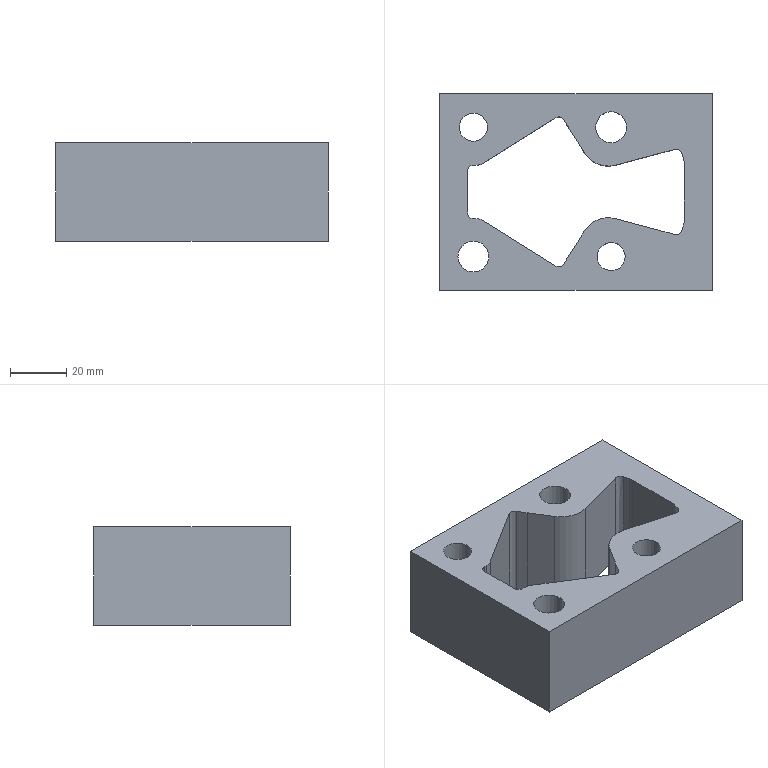Part | NX | features solid 2 | 1 solid | 44 faces | box 97 x 70 x 35 mm | volume 138939 mm3 | plane 20 | cylinder 18 | spline 6 | commonest cylinder face diameters 10 x6 4 x4 11 x2 12 x2 17 x2 20 x2
STEP:
#1=CARTESIAN_POINT('',(1528.396,23.,78.));
#2=VERTEX_POINT('',#1);
#3=CARTESIAN_POINT('',(1533.396,23.,78.));
#4=DIRECTION('',(0.,0.,-1.));
#5=DIRECTION('',(-1.,0.,0.));
#6=AXIS2_PLACEMENT_3D('',#3,#4,#5);
#7=CIRCLE('',#6,5.);
#8=EDGE_CURVE('',#2,#2,#7,.T.);
#9=ORIENTED_EDGE('',*,*,#8,.T.);
#10=EDGE_LOOP('',(#9));
#11=FACE_BOUND('',#10,.T.);
#12=CARTESIAN_POINT('',(1576.896,23.,78.));
#13=VERTEX_POINT('',#12);
#14=CARTESIAN_POINT('',(1582.396,23.,78.));
#15=DIRECTION('',(0.,0.,1.));
#16=DIRECTION('',(-1.,0.,0.));
#17=AXIS2_PLACEMENT_3D('',#14,#15,#16);
#18=CIRCLE('',#17,5.5);
#19=EDGE_CURVE('',#13,#13,#18,.F.);
#20=ORIENTED_EDGE('',*,*,#19,.T.);
#21=EDGE_LOOP('',(#20));
#22=FACE_BOUND('',#21,.T.);
#23=CARTESIAN_POINT('',(1577.396,-23.,78.));
#24=VERTEX_POINT('',#23);
#25=CARTESIAN_POINT('',(1582.396,-23.,78.));
#26=DIRECTION('',(0.,0.,-1.));
#27=DIRECTION('',(-1.,0.,0.));
#28=AXIS2_PLACEMENT_3D('',#25,#26,#27);
#29=CIRCLE('',#28,5.);
#30=EDGE_CURVE('',#24,#24,#29,.T.);
#31=ORIENTED_EDGE('',*,*,#30,.T.);
#32=EDGE_LOOP('',(#31));
#33=FACE_BOUND('',#32,.T.);
#34=CARTESIAN_POINT('',(1538.896,-23.,78.));
#35=VERTEX_POINT('',#34);
#36=CARTESIAN_POINT('',(1533.396,-23.,78.));
#37=DIRECTION('',(0.,0.,1.));
#38=DIRECTION('',(1.,0.,0.));
#39=AXIS2_PLACEMENT_3D('',#36,#37,#38);
#40=CIRCLE('',#39,5.5);
#41=EDGE_CURVE('',#35,#35,#40,.T.);
#42=ORIENTED_EDGE('',*,*,#41,.F.);
#43=EDGE_LOOP('',(#42));
#44=FACE_BOUND('',#43,.T.);
#45=CARTESIAN_POINT('',(1618.396,-35.,78.));
#46=VERTEX_POINT('',#45);
#47=CARTESIAN_POINT('',(1521.396,-35.,78.));
#48=VERTEX_POINT('',#47);
#49=CARTESIAN_POINT('',(1569.896,-35.,78.));
#50=DIRECTION('',(1.,0.,0.));
#51=VECTOR('',#50,1000.);
#52=LINE('',#49,#51);
#53=EDGE_CURVE('',#46,#48,#52,.F.);
#54=ORIENTED_EDGE('',*,*,#53,.F.);
#55=CARTESIAN_POINT('',(1618.396,35.,78.));
#56=VERTEX_POINT('',#55);
#57=CARTESIAN_POINT('',(1618.396,0.,78.));
#58=DIRECTION('',(0.,1.,0.));
#59=VECTOR('',#58,1000.);
#60=LINE('',#57,#59);
#61=EDGE_CURVE('',#56,#46,#60,.F.);
#62=ORIENTED_EDGE('',*,*,#61,.F.);
#63=CARTESIAN_POINT('',(1521.396,35.,78.));
#64=VERTEX_POINT('',#63);
#65=CARTESIAN_POINT('',(1569.896,35.,78.));
#66=DIRECTION('',(-1.,0.,0.));
#67=VECTOR('',#66,1000.);
#68=LINE('',#65,#67);
#69=EDGE_CURVE('',#64,#56,#68,.F.);
#70=ORIENTED_EDGE('',*,*,#69,.F.);
#71=CARTESIAN_POINT('',(1521.396,0.,78.));
#72=DIRECTION('',(0.,-1.,0.));
#73=VECTOR('',#72,1000.);
#74=LINE('',#71,#73);
#75=EDGE_CURVE('',#48,#64,#74,.F.);
#76=ORIENTED_EDGE('',*,*,#75,.F.);
#77=EDGE_LOOP('',(#54,#62,#70,#76));
#78=FACE_BOUND('',#77,.T.);
#79=CARTESIAN_POINT('',(1536.976,-10.26,78.));
#80=VERTEX_POINT('',#79);
#81=CARTESIAN_POINT('',(1534.327,-9.5,78.));
#82=VERTEX_POINT('',#81);
#83=CARTESIAN_POINT('',(1534.327,-14.5,78.));
#84=DIRECTION('',(0.,0.,-1.));
#85=DIRECTION('',(-1.,0.,0.));
#86=AXIS2_PLACEMENT_3D('',#83,#84,#85);
#87=CIRCLE('',#86,5.);
#88=EDGE_CURVE('',#80,#82,#87,.F.);
#89=ORIENTED_EDGE('',*,*,#88,.T.);
#90=CARTESIAN_POINT('',(1533.396,-9.5,78.));
#91=VERTEX_POINT('',#90);
#92=CARTESIAN_POINT('',(984.466,-9.5,78.));
#93=DIRECTION('',(-1.,0.,0.));
#94=VECTOR('',#93,1000.);
#95=LINE('',#92,#94);
#96=EDGE_CURVE('',#82,#91,#95,.T.);
#97=ORIENTED_EDGE('',*,*,#96,.T.);
#98=CARTESIAN_POINT('',(1531.396,-7.5,78.));
#99=VERTEX_POINT('',#98);
#100=CARTESIAN_POINT('',(1533.396,-7.5,78.));
#101=DIRECTION('',(0.,0.,-1.));
#102=DIRECTION('',(-1.,0.,0.));
#103=AXIS2_PLACEMENT_3D('',#100,#101,#102);
#104=CIRCLE('',#103,2.);
#105=EDGE_CURVE('',#91,#99,#104,.T.);
#106=ORIENTED_EDGE('',*,*,#105,.T.);
#107=CARTESIAN_POINT('',(1531.396,7.5,78.));
#108=VERTEX_POINT('',#107);
#109=CARTESIAN_POINT('',(1531.396,0.,78.));
#110=DIRECTION('',(0.,-1.,0.));
#111=VECTOR('',#110,1000.);
#112=LINE('',#109,#111);
#113=EDGE_CURVE('',#108,#99,#112,.T.);
#114=ORIENTED_EDGE('',*,*,#113,.F.);
#115=CARTESIAN_POINT('',(1533.396,9.5,78.));
#116=VERTEX_POINT('',#115);
#117=CARTESIAN_POINT('',(1533.396,7.5,78.));
#118=DIRECTION('',(0.,0.,-1.));
#119=DIRECTION('',(-1.,0.,0.));
#120=AXIS2_PLACEMENT_3D('',#117,#118,#119);
#121=CIRCLE('',#120,2.);
#122=EDGE_CURVE('',#116,#108,#121,.F.);
#123=ORIENTED_EDGE('',*,*,#122,.F.);
#124=CARTESIAN_POINT('',(1534.327,9.5,78.));
#125=VERTEX_POINT('',#124);
#126=CARTESIAN_POINT('',(2186.158,9.5,78.));
#127=DIRECTION('',(-1.,0.,0.));
#128=VECTOR('',#127,1000.);
#129=LINE('',#126,#128);
#130=EDGE_CURVE('',#125,#116,#129,.T.);
#131=ORIENTED_EDGE('',*,*,#130,.F.);
#132=CARTESIAN_POINT('',(1536.976,10.26,78.));
#133=VERTEX_POINT('',#132);
#134=CARTESIAN_POINT('',(1534.327,14.5,78.));
#135=DIRECTION('',(0.,0.,-1.));
#136=DIRECTION('',(-1.,0.,0.));
#137=AXIS2_PLACEMENT_3D('',#134,#135,#136);
#138=CIRCLE('',#137,5.);
#139=EDGE_CURVE('',#133,#125,#138,.T.);
#140=ORIENTED_EDGE('',*,*,#139,.F.);
#141=CARTESIAN_POINT('',(1562.757,26.369,78.));
#142=VERTEX_POINT('',#141);
#143=CARTESIAN_POINT('',(1999.247,299.119,78.));
#144=DIRECTION('',(0.848,0.5299,0.));
#145=VECTOR('',#144,1000.);
#146=LINE('',#143,#145);
#147=EDGE_CURVE('',#142,#133,#146,.F.);
#148=ORIENTED_EDGE('',*,*,#147,.F.);
#149=CARTESIAN_POINT('',(1565.512,25.733,78.));
#150=VERTEX_POINT('',#149);
#151=CARTESIAN_POINT('',(1563.816,24.673,78.));
#152=DIRECTION('',(0.,0.,-1.));
#153=DIRECTION('',(-1.,0.,0.));
#154=AXIS2_PLACEMENT_3D('',#151,#152,#153);
#155=CIRCLE('',#154,2.);
#156=EDGE_CURVE('',#150,#142,#155,.F.);
#157=ORIENTED_EDGE('',*,*,#156,.F.);
#158=CARTESIAN_POINT('',(1567.632,22.341,78.));
#159=VERTEX_POINT('',#158);
#160=CARTESIAN_POINT('',(1567.632,22.341,78.));
#161=DIRECTION('',(-0.5299,0.848,0.));
#162=VECTOR('',#161,1000.);
#163=LINE('',#160,#162);
#164=EDGE_CURVE('',#150,#159,#163,.F.);
#165=ORIENTED_EDGE('',*,*,#164,.T.);
#166=CARTESIAN_POINT('',(1572.931,13.86,78.));
#167=VERTEX_POINT('',#166);
#168=CARTESIAN_POINT('',(1572.931,13.86,78.));
#169=CARTESIAN_POINT('',(1571.165,16.687,78.));
#170=CARTESIAN_POINT('',(1569.399,19.514,78.));
#171=CARTESIAN_POINT('',(1567.632,22.341,78.));
#172=B_SPLINE_CURVE_WITH_KNOTS('',3,(#168,#169,#170,#171),.UNSPECIFIED.,.F.,.F.,(4,4),(0.,0.01),.UNSPECIFIED.);
#173=EDGE_CURVE('',#167,#159,#172,.T.);
#174=ORIENTED_EDGE('',*,*,#173,.F.);
#175=CARTESIAN_POINT('',(1584.,9.5,78.));
#176=VERTEX_POINT('',#175);
#177=CARTESIAN_POINT('',(1581.412,19.159,78.));
#178=DIRECTION('',(0.,0.,-1.));
#179=DIRECTION('',(-1.,0.,0.));
#180=AXIS2_PLACEMENT_3D('',#177,#178,#179);
#181=CIRCLE('',#180,10.);
#182=EDGE_CURVE('',#176,#167,#181,.T.);
#183=ORIENTED_EDGE('',*,*,#182,.F.);
#184=CARTESIAN_POINT('',(1605.133,15.163,78.));
#185=VERTEX_POINT('',#184);
#186=CARTESIAN_POINT('',(1605.133,15.163,78.));
#187=CARTESIAN_POINT('',(1598.089,13.275,78.));
#188=CARTESIAN_POINT('',(1591.044,11.388,78.));
#189=CARTESIAN_POINT('',(1584.,9.5,78.));
#190=B_SPLINE_CURVE_WITH_KNOTS('',3,(#186,#187,#188,#189),.UNSPECIFIED.,.F.,.F.,(4,4),(0.,0.02188),.UNSPECIFIED.);
#191=EDGE_CURVE('',#185,#176,#190,.T.);
#192=ORIENTED_EDGE('',*,*,#191,.F.);
#193=CARTESIAN_POINT('',(1607.583,13.748,78.));
#194=VERTEX_POINT('',#193);
#195=CARTESIAN_POINT('',(1605.651,13.231,78.));
#196=DIRECTION('',(0.,0.,-1.));
#197=DIRECTION('',(-1.,0.,0.));
#198=AXIS2_PLACEMENT_3D('',#195,#196,#197);
#199=CIRCLE('',#198,2.);
#200=EDGE_CURVE('',#194,#185,#199,.F.);
#201=ORIENTED_EDGE('',*,*,#200,.F.);
#202=CARTESIAN_POINT('',(1608.226,11.348,78.));
#203=VERTEX_POINT('',#202);
#204=CARTESIAN_POINT('',(1602.079,34.289,78.));
#205=DIRECTION('',(-0.2588,0.9659,0.));
#206=VECTOR('',#205,1000.);
#207=LINE('',#204,#206);
#208=EDGE_CURVE('',#194,#203,#207,.F.);
#209=ORIENTED_EDGE('',*,*,#208,.T.);
#210=CARTESIAN_POINT('',(1608.396,10.054,78.));
#211=VERTEX_POINT('',#210);
#212=CARTESIAN_POINT('',(1603.396,10.054,78.));
#213=DIRECTION('',(0.,0.,-1.));
#214=DIRECTION('',(-1.,0.,0.));
#215=AXIS2_PLACEMENT_3D('',#212,#213,#214);
#216=CIRCLE('',#215,5.);
#217=EDGE_CURVE('',#211,#203,#216,.F.);
#218=ORIENTED_EDGE('',*,*,#217,.F.);
#219=CARTESIAN_POINT('',(1608.396,-10.054,78.));
#220=VERTEX_POINT('',#219);
#221=CARTESIAN_POINT('',(1608.396,-4.33,78.));
#222=DIRECTION('',(0.,-1.,0.));
#223=VECTOR('',#222,1000.);
#224=LINE('',#221,#223);
#225=EDGE_CURVE('',#220,#211,#224,.F.);
#226=ORIENTED_EDGE('',*,*,#225,.F.);
#227=CARTESIAN_POINT('',(1608.226,-11.348,78.));
#228=VERTEX_POINT('',#227);
#229=CARTESIAN_POINT('',(1603.396,-10.054,78.));
#230=DIRECTION('',(0.,0.,-1.));
#231=DIRECTION('',(-1.,0.,0.));
#232=AXIS2_PLACEMENT_3D('',#229,#230,#231);
#233=CIRCLE('',#232,5.);
#234=EDGE_CURVE('',#220,#228,#233,.T.);
#235=ORIENTED_EDGE('',*,*,#234,.T.);
#236=CARTESIAN_POINT('',(1607.583,-13.748,78.));
#237=VERTEX_POINT('',#236);
#238=CARTESIAN_POINT('',(1602.079,-34.289,78.));
#239=DIRECTION('',(0.2588,0.9659,0.));
#240=VECTOR('',#239,1000.);
#241=LINE('',#238,#240);
#242=EDGE_CURVE('',#228,#237,#241,.F.);
#243=ORIENTED_EDGE('',*,*,#242,.T.);
#244=CARTESIAN_POINT('',(1605.133,-15.163,78.));
#245=VERTEX_POINT('',#244);
#246=CARTESIAN_POINT('',(1605.651,-13.231,78.));
#247=DIRECTION('',(0.,0.,-1.));
#248=DIRECTION('',(-1.,0.,0.));
#249=AXIS2_PLACEMENT_3D('',#246,#247,#248);
#250=CIRCLE('',#249,2.);
#251=EDGE_CURVE('',#237,#245,#250,.T.);
#252=ORIENTED_EDGE('',*,*,#251,.T.);
#253=CARTESIAN_POINT('',(1584.,-9.5,78.));
#254=VERTEX_POINT('',#253);
#255=CARTESIAN_POINT('',(1605.133,-15.163,78.));
#256=CARTESIAN_POINT('',(1598.089,-13.275,78.));
#257=CARTESIAN_POINT('',(1591.044,-11.388,78.));
#258=CARTESIAN_POINT('',(1584.,-9.5,78.));
#259=B_SPLINE_CURVE_WITH_KNOTS('',3,(#255,#256,#257,#258),.UNSPECIFIED.,.F.,.F.,(4,4),(0.,0.02188),.UNSPECIFIED.);
#260=EDGE_CURVE('',#245,#254,#259,.T.);
#261=ORIENTED_EDGE('',*,*,#260,.T.);
#262=CARTESIAN_POINT('',(1572.931,-13.86,78.));
#263=VERTEX_POINT('',#262);
#264=CARTESIAN_POINT('',(1581.412,-19.159,78.));
#265=DIRECTION('',(0.,0.,-1.));
#266=DIRECTION('',(-1.,0.,0.));
#267=AXIS2_PLACEMENT_3D('',#264,#265,#266);
#268=CIRCLE('',#267,10.);
#269=EDGE_CURVE('',#254,#263,#268,.F.);
#270=ORIENTED_EDGE('',*,*,#269,.T.);
#271=CARTESIAN_POINT('',(1567.632,-22.341,78.));
#272=VERTEX_POINT('',#271);
#273=CARTESIAN_POINT('',(1572.931,-13.86,78.));
#274=CARTESIAN_POINT('',(1571.165,-16.687,78.));
#275=CARTESIAN_POINT('',(1569.399,-19.514,78.));
#276=CARTESIAN_POINT('',(1567.632,-22.341,78.));
#277=B_SPLINE_CURVE_WITH_KNOTS('',3,(#273,#274,#275,#276),.UNSPECIFIED.,.F.,.F.,(4,4),(0.,0.01),.UNSPECIFIED.);
#278=EDGE_CURVE('',#263,#272,#277,.T.);
#279=ORIENTED_EDGE('',*,*,#278,.T.);
#280=CARTESIAN_POINT('',(1565.512,-25.733,78.));
#281=VERTEX_POINT('',#280);
#282=CARTESIAN_POINT('',(1751.363,271.69,78.));
#283=DIRECTION('',(-0.5299,-0.848,0.));
#284=VECTOR('',#283,1000.);
#285=LINE('',#282,#284);
#286=EDGE_CURVE('',#281,#272,#285,.F.);
#287=ORIENTED_EDGE('',*,*,#286,.F.);
#288=CARTESIAN_POINT('',(1562.757,-26.369,78.));
#289=VERTEX_POINT('',#288);
#290=CARTESIAN_POINT('',(1563.816,-24.673,78.));
#291=DIRECTION('',(0.,0.,-1.));
#292=DIRECTION('',(-1.,0.,0.));
#293=AXIS2_PLACEMENT_3D('',#290,#291,#292);
#294=CIRCLE('',#293,2.);
#295=EDGE_CURVE('',#281,#289,#294,.T.);
#296=ORIENTED_EDGE('',*,*,#295,.T.);
#297=CARTESIAN_POINT('',(1636.537,-72.472,78.));
#298=DIRECTION('',(0.848,-0.5299,0.));
#299=VECTOR('',#298,1000.);
#300=LINE('',#297,#299);
#301=EDGE_CURVE('',#289,#80,#300,.F.);
#302=ORIENTED_EDGE('',*,*,#301,.T.);
#303=EDGE_LOOP('',(#89,#97,#106,#114,#123,#131,#140,#148,#157,#165,#174,#183,#192,#201,#209,#218,#226,#235,#243,#252,#261,#270,#279,#287,#296,#302));
#304=FACE_BOUND('',#303,.T.);
#305=CARTESIAN_POINT('',(2186.158,0.000000688,78.));
#306=DIRECTION('',(0.,0.,-1.));
#307=DIRECTION('',(1.,0.,0.));
#308=AXIS2_PLACEMENT_3D('',#305,#306,#307);
#309=PLANE('',#308);
#310=ADVANCED_FACE('',(#11,#22,#33,#44,#78,#304),#309,.F.);
#311=CARTESIAN_POINT('',(1527.396,23.,43.));
#312=VERTEX_POINT('',#311);
#313=CARTESIAN_POINT('',(1533.396,23.,43.));
#314=DIRECTION('',(0.,0.,-1.));
#315=DIRECTION('',(-1.,0.,0.));
#316=AXIS2_PLACEMENT_3D('',#313,#314,#315);
#317=CIRCLE('',#316,6.);
#318=EDGE_CURVE('',#312,#312,#317,.F.);
#319=ORIENTED_EDGE('',*,*,#318,.F.);
#320=EDGE_LOOP('',(#319));
#321=FACE_BOUND('',#320,.T.);
#322=CARTESIAN_POINT('',(1539.396,23.,58.));
#323=VERTEX_POINT('',#322);
#324=CARTESIAN_POINT('',(1533.396,23.,58.));
#325=DIRECTION('',(0.,0.,1.));
#326=DIRECTION('',(1.,0.,0.));
#327=AXIS2_PLACEMENT_3D('',#324,#325,#326);
#328=CIRCLE('',#327,6.);
#329=EDGE_CURVE('',#323,#323,#328,.F.);
#330=ORIENTED_EDGE('',*,*,#329,.F.);
#331=EDGE_LOOP('',(#330));
#332=FACE_BOUND('',#331,.T.);
#333=CARTESIAN_POINT('',(1533.396,23.,43.));
#334=DIRECTION('',(0.,0.,1.));
#335=DIRECTION('',(1.,0.,0.));
#336=AXIS2_PLACEMENT_3D('',#333,#334,#335);
#337=CYLINDRICAL_SURFACE('',#336,6.);
#338=ADVANCED_FACE('',(#321,#332),#337,.F.);
#339=ORIENTED_EDGE('',*,*,#8,.F.);
#340=EDGE_LOOP('',(#339));
#341=FACE_BOUND('',#340,.T.);
#342=CARTESIAN_POINT('',(1538.396,23.,58.));
#343=VERTEX_POINT('',#342);
#344=CARTESIAN_POINT('',(1533.396,23.,58.));
#345=DIRECTION('',(0.,0.,1.));
#346=DIRECTION('',(1.,0.,0.));
#347=AXIS2_PLACEMENT_3D('',#344,#345,#346);
#348=CIRCLE('',#347,5.);
#349=EDGE_CURVE('',#343,#343,#348,.F.);
#350=ORIENTED_EDGE('',*,*,#349,.T.);
#351=EDGE_LOOP('',(#350));
#352=FACE_BOUND('',#351,.T.);
#353=CARTESIAN_POINT('',(1533.396,23.,78.));
#354=DIRECTION('',(0.,0.,1.));
#355=DIRECTION('',(1.,0.,0.));
#356=AXIS2_PLACEMENT_3D('',#353,#354,#355);
#357=CYLINDRICAL_SURFACE('',#356,5.);
#358=ADVANCED_FACE('',(#341,#352),#357,.F.);
#359=ORIENTED_EDGE('',*,*,#329,.T.);
#360=EDGE_LOOP('',(#359));
#361=FACE_BOUND('',#360,.T.);
#362=ORIENTED_EDGE('',*,*,#349,.F.);
#363=EDGE_LOOP('',(#362));
#364=FACE_BOUND('',#363,.T.);
#365=CARTESIAN_POINT('',(1531.574,23.49,58.));
#366=DIRECTION('',(0.,0.,1.));
#367=DIRECTION('',(1.,0.,0.));
#368=AXIS2_PLACEMENT_3D('',#365,#366,#367);
#369=PLANE('',#368);
#370=ADVANCED_FACE('',(#361,#364),#369,.F.);
#371=CARTESIAN_POINT('',(1573.896,23.,43.));
#372=VERTEX_POINT('',#371);
#373=CARTESIAN_POINT('',(1582.396,23.,43.));
#374=DIRECTION('',(0.,0.,1.));
#375=DIRECTION('',(-1.,0.,0.));
#376=AXIS2_PLACEMENT_3D('',#373,#374,#375);
#377=CIRCLE('',#376,8.5);
#378=EDGE_CURVE('',#372,#372,#377,.T.);
#379=ORIENTED_EDGE('',*,*,#378,.F.);
#380=EDGE_LOOP('',(#379));
#381=FACE_BOUND('',#380,.T.);
#382=CARTESIAN_POINT('',(1573.896,23.,58.));
#383=VERTEX_POINT('',#382);
#384=CARTESIAN_POINT('',(1582.396,23.,58.));
#385=DIRECTION('',(0.,0.,1.));
#386=DIRECTION('',(-1.,0.,0.));
#387=AXIS2_PLACEMENT_3D('',#384,#385,#386);
#388=CIRCLE('',#387,8.5);
#389=EDGE_CURVE('',#383,#383,#388,.F.);
#390=ORIENTED_EDGE('',*,*,#389,.F.);
#391=EDGE_LOOP('',(#390));
#392=FACE_BOUND('',#391,.T.);
#393=CARTESIAN_POINT('',(1582.396,23.,43.));
#394=DIRECTION('',(0.,0.,1.));
#395=DIRECTION('',(-1.,0.,0.));
#396=AXIS2_PLACEMENT_3D('',#393,#394,#395);
#397=CYLINDRICAL_SURFACE('',#396,8.5);
#398=ADVANCED_FACE('',(#381,#392),#397,.F.);
#399=ORIENTED_EDGE('',*,*,#19,.F.);
#400=EDGE_LOOP('',(#399));
#401=FACE_BOUND('',#400,.T.);
#402=CARTESIAN_POINT('',(1576.896,23.,58.));
#403=VERTEX_POINT('',#402);
#404=CARTESIAN_POINT('',(1582.396,23.,58.));
#405=DIRECTION('',(0.,0.,1.));
#406=DIRECTION('',(-1.,0.,0.));
#407=AXIS2_PLACEMENT_3D('',#404,#405,#406);
#408=CIRCLE('',#407,5.5);
#409=EDGE_CURVE('',#403,#403,#408,.F.);
#410=ORIENTED_EDGE('',*,*,#409,.T.);
#411=EDGE_LOOP('',(#410));
#412=FACE_BOUND('',#411,.T.);
#413=CARTESIAN_POINT('',(1582.396,23.,78.));
#414=DIRECTION('',(0.,0.,1.));
#415=DIRECTION('',(-1.,0.,0.));
#416=AXIS2_PLACEMENT_3D('',#413,#414,#415);
#417=CYLINDRICAL_SURFACE('',#416,5.5);
#418=ADVANCED_FACE('',(#401,#412),#417,.F.);
#419=ORIENTED_EDGE('',*,*,#389,.T.);
#420=EDGE_LOOP('',(#419));
#421=FACE_BOUND('',#420,.T.);
#422=ORIENTED_EDGE('',*,*,#409,.F.);
#423=EDGE_LOOP('',(#422));
#424=FACE_BOUND('',#423,.T.);
#425=CARTESIAN_POINT('',(1584.218,23.49,58.));
#426=DIRECTION('',(0.,0.,1.));
#427=DIRECTION('',(-1.,0.,0.));
#428=AXIS2_PLACEMENT_3D('',#425,#426,#427);
#429=PLANE('',#428);
#430=ADVANCED_FACE('',(#421,#424),#429,.F.);
#431=CARTESIAN_POINT('',(1541.896,-23.,58.));
#432=VERTEX_POINT('',#431);
#433=CARTESIAN_POINT('',(1533.396,-23.,58.));
#434=DIRECTION('',(0.,0.,1.));
#435=DIRECTION('',(1.,0.,0.));
#436=AXIS2_PLACEMENT_3D('',#433,#434,#435);
#437=CIRCLE('',#436,8.5);
#438=EDGE_CURVE('',#432,#432,#437,.F.);
#439=ORIENTED_EDGE('',*,*,#438,.T.);
#440=EDGE_LOOP('',(#439));
#441=FACE_BOUND('',#440,.T.);
#442=CARTESIAN_POINT('',(1538.896,-23.,58.));
#443=VERTEX_POINT('',#442);
#444=CARTESIAN_POINT('',(1533.396,-23.,58.));
#445=DIRECTION('',(0.,0.,1.));
#446=DIRECTION('',(1.,0.,0.));
#447=AXIS2_PLACEMENT_3D('',#444,#445,#446);
#448=CIRCLE('',#447,5.5);
#449=EDGE_CURVE('',#443,#443,#448,.F.);
#450=ORIENTED_EDGE('',*,*,#449,.F.);
#451=EDGE_LOOP('',(#450));
#452=FACE_BOUND('',#451,.T.);
#453=CARTESIAN_POINT('',(1531.574,-23.49,58.));
#454=DIRECTION('',(0.,0.,1.));
#455=DIRECTION('',(1.,0.,0.));
#456=AXIS2_PLACEMENT_3D('',#453,#454,#455);
#457=PLANE('',#456);
#458=ADVANCED_FACE('',(#441,#452),#457,.F.);
#459=CARTESIAN_POINT('',(1588.396,-23.,58.));
#460=VERTEX_POINT('',#459);
#461=CARTESIAN_POINT('',(1582.396,-23.,58.));
#462=DIRECTION('',(0.,0.,1.));
#463=DIRECTION('',(1.,0.,0.));
#464=AXIS2_PLACEMENT_3D('',#461,#462,#463);
#465=CIRCLE('',#464,6.);
#466=EDGE_CURVE('',#460,#460,#465,.F.);
#467=ORIENTED_EDGE('',*,*,#466,.T.);
#468=EDGE_LOOP('',(#467));
#469=FACE_BOUND('',#468,.T.);
#470=CARTESIAN_POINT('',(1587.396,-23.,58.));
#471=VERTEX_POINT('',#470);
#472=CARTESIAN_POINT('',(1582.396,-23.,58.));
#473=DIRECTION('',(0.,0.,1.));
#474=DIRECTION('',(1.,0.,0.));
#475=AXIS2_PLACEMENT_3D('',#472,#473,#474);
#476=CIRCLE('',#475,5.);
#477=EDGE_CURVE('',#471,#471,#476,.F.);
#478=ORIENTED_EDGE('',*,*,#477,.F.);
#479=EDGE_LOOP('',(#478));
#480=FACE_BOUND('',#479,.T.);
#481=CARTESIAN_POINT('',(1584.218,-23.49,58.));
#482=DIRECTION('',(0.,0.,1.));
#483=DIRECTION('',(-1.,0.,0.));
#484=AXIS2_PLACEMENT_3D('',#481,#482,#483);
#485=PLANE('',#484);
#486=ADVANCED_FACE('',(#469,#480),#485,.F.);
#487=CARTESIAN_POINT('',(1541.896,-23.,43.));
#488=VERTEX_POINT('',#487);
#489=CARTESIAN_POINT('',(1533.396,-23.,43.));
#490=DIRECTION('',(0.,0.,1.));
#491=DIRECTION('',(1.,0.,0.));
#492=AXIS2_PLACEMENT_3D('',#489,#490,#491);
#493=CIRCLE('',#492,8.5);
#494=EDGE_CURVE('',#488,#488,#493,.T.);
#495=ORIENTED_EDGE('',*,*,#494,.F.);
#496=EDGE_LOOP('',(#495));
#497=FACE_BOUND('',#496,.T.);
#498=ORIENTED_EDGE('',*,*,#438,.F.);
#499=EDGE_LOOP('',(#498));
#500=FACE_BOUND('',#499,.T.);
#501=CARTESIAN_POINT('',(1533.396,-23.,43.));
#502=DIRECTION('',(0.,0.,1.));
#503=DIRECTION('',(1.,0.,0.));
#504=AXIS2_PLACEMENT_3D('',#501,#502,#503);
#505=CYLINDRICAL_SURFACE('',#504,8.5);
#506=ADVANCED_FACE('',(#497,#500),#505,.F.);
#507=CARTESIAN_POINT('',(1521.396,-35.,43.));
#508=VERTEX_POINT('',#507);
#509=CARTESIAN_POINT('',(1521.396,-35.,22.));
#510=DIRECTION('',(0.,0.,1.));
#511=VECTOR('',#510,1000.);
#512=LINE('',#509,#511);
#513=EDGE_CURVE('',#508,#48,#512,.T.);
#514=ORIENTED_EDGE('',*,*,#513,.T.);
#515=ORIENTED_EDGE('',*,*,#75,.T.);
#516=CARTESIAN_POINT('',(1521.396,35.,43.));
#517=VERTEX_POINT('',#516);
#518=CARTESIAN_POINT('',(1521.396,35.,22.));
#519=DIRECTION('',(0.,0.,1.));
#520=VECTOR('',#519,1000.);
#521=LINE('',#518,#520);
#522=EDGE_CURVE('',#517,#64,#521,.T.);
#523=ORIENTED_EDGE('',*,*,#522,.F.);
#524=CARTESIAN_POINT('',(1521.396,0.,43.));
#525=DIRECTION('',(0.,-1.,0.));
#526=VECTOR('',#525,1000.);
#527=LINE('',#524,#526);
#528=EDGE_CURVE('',#517,#508,#527,.T.);
#529=ORIENTED_EDGE('',*,*,#528,.T.);
#530=EDGE_LOOP('',(#514,#515,#523,#529));
#531=FACE_BOUND('',#530,.T.);
#532=CARTESIAN_POINT('',(1521.396,0.,22.));
#533=DIRECTION('',(-1.,0.,0.));
#534=DIRECTION('',(0.,0.,1.));
#535=AXIS2_PLACEMENT_3D('',#532,#533,#534);
#536=PLANE('',#535);
#537=ADVANCED_FACE('',(#531),#536,.T.);
#538=ORIENTED_EDGE('',*,*,#522,.T.);
#539=ORIENTED_EDGE('',*,*,#69,.T.);
#540=CARTESIAN_POINT('',(1618.396,35.,43.));
#541=VERTEX_POINT('',#540);
#542=CARTESIAN_POINT('',(1618.396,35.,22.));
#543=DIRECTION('',(0.,0.,1.));
#544=VECTOR('',#543,1000.);
#545=LINE('',#542,#544);
#546=EDGE_CURVE('',#541,#56,#545,.T.);
#547=ORIENTED_EDGE('',*,*,#546,.F.);
#548=CARTESIAN_POINT('',(1569.896,35.,43.));
#549=DIRECTION('',(-1.,0.,0.));
#550=VECTOR('',#549,1000.);
#551=LINE('',#548,#550);
#552=EDGE_CURVE('',#541,#517,#551,.T.);
#553=ORIENTED_EDGE('',*,*,#552,.T.);
#554=EDGE_LOOP('',(#538,#539,#547,#553));
#555=FACE_BOUND('',#554,.T.);
#556=CARTESIAN_POINT('',(1569.896,35.,22.));
#557=DIRECTION('',(0.,1.,0.));
#558=DIRECTION('',(0.,0.,1.));
#559=AXIS2_PLACEMENT_3D('',#556,#557,#558);
#560=PLANE('',#559);
#561=ADVANCED_FACE('',(#555),#560,.T.);
#562=CARTESIAN_POINT('',(1618.396,-35.,43.));
#563=VERTEX_POINT('',#562);
#564=CARTESIAN_POINT('',(1618.396,0.,43.));
#565=DIRECTION('',(0.,1.,0.));
#566=VECTOR('',#565,1000.);
#567=LINE('',#564,#566);
#568=EDGE_CURVE('',#563,#541,#567,.T.);
#569=ORIENTED_EDGE('',*,*,#568,.T.);
#570=ORIENTED_EDGE('',*,*,#546,.T.);
#571=ORIENTED_EDGE('',*,*,#61,.T.);
#572=CARTESIAN_POINT('',(1618.396,-35.,22.));
#573=DIRECTION('',(0.,0.,1.));
#574=VECTOR('',#573,1000.);
#575=LINE('',#572,#574);
#576=EDGE_CURVE('',#563,#46,#575,.T.);
#577=ORIENTED_EDGE('',*,*,#576,.F.);
#578=EDGE_LOOP('',(#569,#570,#571,#577));
#579=FACE_BOUND('',#578,.T.);
#580=CARTESIAN_POINT('',(1618.396,0.,22.));
#581=DIRECTION('',(1.,0.,0.));
#582=DIRECTION('',(0.,0.,-1.));
#583=AXIS2_PLACEMENT_3D('',#580,#581,#582);
#584=PLANE('',#583);
#585=ADVANCED_FACE('',(#579),#584,.T.);
#586=ORIENTED_EDGE('',*,*,#513,.F.);
#587=CARTESIAN_POINT('',(1569.896,-35.,43.));
#588=DIRECTION('',(1.,0.,0.));
#589=VECTOR('',#588,1000.);
#590=LINE('',#587,#589);
#591=EDGE_CURVE('',#508,#563,#590,.T.);
#592=ORIENTED_EDGE('',*,*,#591,.T.);
#593=ORIENTED_EDGE('',*,*,#576,.T.);
#594=ORIENTED_EDGE('',*,*,#53,.T.);
#595=EDGE_LOOP('',(#586,#592,#593,#594));
#596=FACE_BOUND('',#595,.T.);
#597=CARTESIAN_POINT('',(1569.896,-35.,22.));
#598=DIRECTION('',(0.,-1.,0.));
#599=DIRECTION('',(0.,0.,-1.));
#600=AXIS2_PLACEMENT_3D('',#597,#598,#599);
#601=PLANE('',#600);
#602=ADVANCED_FACE('',(#596),#601,.T.);
#603=ORIENTED_EDGE('',*,*,#41,.T.);
#604=EDGE_LOOP('',(#603));
#605=FACE_BOUND('',#604,.T.);
#606=ORIENTED_EDGE('',*,*,#449,.T.);
#607=EDGE_LOOP('',(#606));
#608=FACE_BOUND('',#607,.T.);
#609=CARTESIAN_POINT('',(1533.396,-23.,78.));
#610=DIRECTION('',(0.,0.,1.));
#611=DIRECTION('',(1.,0.,0.));
#612=AXIS2_PLACEMENT_3D('',#609,#610,#611);
#613=CYLINDRICAL_SURFACE('',#612,5.5);
#614=ADVANCED_FACE('',(#605,#608),#613,.F.);
#615=ORIENTED_EDGE('',*,*,#30,.F.);
#616=EDGE_LOOP('',(#615));
#617=FACE_BOUND('',#616,.T.);
#618=ORIENTED_EDGE('',*,*,#477,.T.);
#619=EDGE_LOOP('',(#618));
#620=FACE_BOUND('',#619,.T.);
#621=CARTESIAN_POINT('',(1582.396,-23.,78.));
#622=DIRECTION('',(0.,0.,1.));
#623=DIRECTION('',(-1.,0.,0.));
#624=AXIS2_PLACEMENT_3D('',#621,#622,#623);
#625=CYLINDRICAL_SURFACE('',#624,5.);
#626=ADVANCED_FACE('',(#617,#620),#625,.F.);
#627=CARTESIAN_POINT('',(1576.396,-23.,43.));
#628=VERTEX_POINT('',#627);
#629=CARTESIAN_POINT('',(1582.396,-23.,43.));
#630=DIRECTION('',(0.,0.,-1.));
#631=DIRECTION('',(-1.,0.,0.));
#632=AXIS2_PLACEMENT_3D('',#629,#630,#631);
#633=CIRCLE('',#632,6.);
#634=EDGE_CURVE('',#628,#628,#633,.F.);
#635=ORIENTED_EDGE('',*,*,#634,.F.);
#636=EDGE_LOOP('',(#635));
#637=FACE_BOUND('',#636,.T.);
#638=ORIENTED_EDGE('',*,*,#466,.F.);
#639=EDGE_LOOP('',(#638));
#640=FACE_BOUND('',#639,.T.);
#641=CARTESIAN_POINT('',(1582.396,-23.,43.));
#642=DIRECTION('',(0.,0.,1.));
#643=DIRECTION('',(-1.,0.,0.));
#644=AXIS2_PLACEMENT_3D('',#641,#642,#643);
#645=CYLINDRICAL_SURFACE('',#644,6.);
#646=ADVANCED_FACE('',(#637,#640),#645,.F.);
#647=CARTESIAN_POINT('',(1533.396,-9.5,43.));
#648=VERTEX_POINT('',#647);
#649=CARTESIAN_POINT('',(1531.396,-7.5,43.));
#650=VERTEX_POINT('',#649);
#651=CARTESIAN_POINT('',(1533.396,-7.5,43.));
#652=DIRECTION('',(0.,0.,-1.));
#653=DIRECTION('',(-1.,0.,0.));
#654=AXIS2_PLACEMENT_3D('',#651,#652,#653);
#655=CIRCLE('',#654,2.);
#656=EDGE_CURVE('',#648,#650,#655,.T.);
#657=ORIENTED_EDGE('',*,*,#656,.F.);
#658=CARTESIAN_POINT('',(1534.327,-9.5,43.));
#659=VERTEX_POINT('',#658);
#660=CARTESIAN_POINT('',(1385.079,-9.5,43.));
#661=DIRECTION('',(1.,0.,0.));
#662=VECTOR('',#661,1000.);
#663=LINE('',#660,#662);
#664=EDGE_CURVE('',#659,#648,#663,.F.);
#665=ORIENTED_EDGE('',*,*,#664,.F.);
#666=CARTESIAN_POINT('',(1536.976,-10.26,43.));
#667=VERTEX_POINT('',#666);
#668=CARTESIAN_POINT('',(1534.327,-14.5,43.));
#669=DIRECTION('',(0.,0.,-1.));
#670=DIRECTION('',(-1.,0.,0.));
#671=AXIS2_PLACEMENT_3D('',#668,#669,#670);
#672=CIRCLE('',#671,5.);
#673=EDGE_CURVE('',#659,#667,#672,.T.);
#674=ORIENTED_EDGE('',*,*,#673,.T.);
#675=CARTESIAN_POINT('',(1562.757,-26.369,43.));
#676=VERTEX_POINT('',#675);
#677=CARTESIAN_POINT('',(1359.352,100.732,43.));
#678=DIRECTION('',(-0.848,0.5299,0.));
#679=VECTOR('',#678,1000.);
#680=LINE('',#677,#679);
#681=EDGE_CURVE('',#676,#667,#680,.T.);
#682=ORIENTED_EDGE('',*,*,#681,.F.);
#683=CARTESIAN_POINT('',(1565.512,-25.733,43.));
#684=VERTEX_POINT('',#683);
#685=CARTESIAN_POINT('',(1563.816,-24.673,43.));
#686=DIRECTION('',(0.,0.,-1.));
#687=DIRECTION('',(-1.,0.,0.));
#688=AXIS2_PLACEMENT_3D('',#685,#686,#687);
#689=CIRCLE('',#688,2.);
#690=EDGE_CURVE('',#684,#676,#689,.T.);
#691=ORIENTED_EDGE('',*,*,#690,.F.);
#692=CARTESIAN_POINT('',(1567.632,-22.341,43.));
#693=VERTEX_POINT('',#692);
#694=CARTESIAN_POINT('',(1590.18,13.743,43.));
#695=DIRECTION('',(-0.5299,-0.848,0.));
#696=VECTOR('',#695,1000.);
#697=LINE('',#694,#696);
#698=EDGE_CURVE('',#693,#684,#697,.T.);
#699=ORIENTED_EDGE('',*,*,#698,.F.);
#700=CARTESIAN_POINT('',(1572.931,-13.86,43.));
#701=VERTEX_POINT('',#700);
#702=CARTESIAN_POINT('',(1567.632,-22.341,43.));
#703=CARTESIAN_POINT('',(1569.399,-19.514,43.));
#704=CARTESIAN_POINT('',(1571.165,-16.687,43.));
#705=CARTESIAN_POINT('',(1572.931,-13.86,43.));
#706=B_SPLINE_CURVE_WITH_KNOTS('',3,(#702,#703,#704,#705),.UNSPECIFIED.,.F.,.F.,(4,4),(0.,0.01),.UNSPECIFIED.);
#707=EDGE_CURVE('',#693,#701,#706,.T.);
#708=ORIENTED_EDGE('',*,*,#707,.T.);
#709=CARTESIAN_POINT('',(1584.,-9.5,43.));
#710=VERTEX_POINT('',#709);
#711=CARTESIAN_POINT('',(1581.412,-19.159,43.));
#712=DIRECTION('',(0.,0.,-1.));
#713=DIRECTION('',(-1.,0.,0.));
#714=AXIS2_PLACEMENT_3D('',#711,#712,#713);
#715=CIRCLE('',#714,10.);
#716=EDGE_CURVE('',#701,#710,#715,.T.);
#717=ORIENTED_EDGE('',*,*,#716,.T.);
#718=CARTESIAN_POINT('',(1605.133,-15.163,43.));
#719=VERTEX_POINT('',#718);
#720=CARTESIAN_POINT('',(1584.,-9.5,43.));
#721=CARTESIAN_POINT('',(1591.044,-11.388,43.));
#722=CARTESIAN_POINT('',(1598.089,-13.275,43.));
#723=CARTESIAN_POINT('',(1605.133,-15.163,43.));
#724=B_SPLINE_CURVE_WITH_KNOTS('',3,(#720,#721,#722,#723),.UNSPECIFIED.,.F.,.F.,(4,4),(0.,0.02188),.UNSPECIFIED.);
#725=EDGE_CURVE('',#710,#719,#724,.T.);
#726=ORIENTED_EDGE('',*,*,#725,.T.);
#727=CARTESIAN_POINT('',(1607.583,-13.748,43.));
#728=VERTEX_POINT('',#727);
#729=CARTESIAN_POINT('',(1605.651,-13.231,43.));
#730=DIRECTION('',(0.,0.,-1.));
#731=DIRECTION('',(-1.,0.,0.));
#732=AXIS2_PLACEMENT_3D('',#729,#730,#731);
#733=CIRCLE('',#732,2.);
#734=EDGE_CURVE('',#728,#719,#733,.T.);
#735=ORIENTED_EDGE('',*,*,#734,.F.);
#736=CARTESIAN_POINT('',(1608.226,-11.348,43.));
#737=VERTEX_POINT('',#736);
#738=CARTESIAN_POINT('',(1631.591,75.851,43.));
#739=DIRECTION('',(-0.2588,-0.9659,0.));
#740=VECTOR('',#739,1000.);
#741=LINE('',#738,#740);
#742=EDGE_CURVE('',#737,#728,#741,.T.);
#743=ORIENTED_EDGE('',*,*,#742,.F.);
#744=CARTESIAN_POINT('',(1608.396,-10.054,43.));
#745=VERTEX_POINT('',#744);
#746=CARTESIAN_POINT('',(1603.396,-10.054,43.));
#747=DIRECTION('',(0.,0.,-1.));
#748=DIRECTION('',(-1.,0.,0.));
#749=AXIS2_PLACEMENT_3D('',#746,#747,#748);
#750=CIRCLE('',#749,5.);
#751=EDGE_CURVE('',#745,#737,#750,.T.);
#752=ORIENTED_EDGE('',*,*,#751,.F.);
#753=CARTESIAN_POINT('',(1608.396,10.054,43.));
#754=VERTEX_POINT('',#753);
#755=CARTESIAN_POINT('',(1608.396,141.904,43.));
#756=DIRECTION('',(0.,1.,0.));
#757=VECTOR('',#756,1000.);
#758=LINE('',#755,#757);
#759=EDGE_CURVE('',#745,#754,#758,.T.);
#760=ORIENTED_EDGE('',*,*,#759,.T.);
#761=CARTESIAN_POINT('',(1608.226,11.348,43.));
#762=VERTEX_POINT('',#761);
#763=CARTESIAN_POINT('',(1603.396,10.054,43.));
#764=DIRECTION('',(0.,0.,-1.));
#765=DIRECTION('',(-1.,0.,0.));
#766=AXIS2_PLACEMENT_3D('',#763,#764,#765);
#767=CIRCLE('',#766,5.);
#768=EDGE_CURVE('',#762,#754,#767,.T.);
#769=ORIENTED_EDGE('',*,*,#768,.F.);
#770=CARTESIAN_POINT('',(1607.583,13.748,43.));
#771=VERTEX_POINT('',#770);
#772=CARTESIAN_POINT('',(1560.639,188.945,43.));
#773=DIRECTION('',(0.2588,-0.9659,0.));
#774=VECTOR('',#773,1000.);
#775=LINE('',#772,#774);
#776=EDGE_CURVE('',#771,#762,#775,.T.);
#777=ORIENTED_EDGE('',*,*,#776,.F.);
#778=CARTESIAN_POINT('',(1605.133,15.163,43.));
#779=VERTEX_POINT('',#778);
#780=CARTESIAN_POINT('',(1605.651,13.231,43.));
#781=DIRECTION('',(0.,0.,-1.));
#782=DIRECTION('',(-1.,0.,0.));
#783=AXIS2_PLACEMENT_3D('',#780,#781,#782);
#784=CIRCLE('',#783,2.);
#785=EDGE_CURVE('',#779,#771,#784,.T.);
#786=ORIENTED_EDGE('',*,*,#785,.F.);
#787=CARTESIAN_POINT('',(1584.,9.5,43.));
#788=VERTEX_POINT('',#787);
#789=CARTESIAN_POINT('',(1605.133,15.163,43.));
#790=CARTESIAN_POINT('',(1598.089,13.275,43.));
#791=CARTESIAN_POINT('',(1591.044,11.388,43.));
#792=CARTESIAN_POINT('',(1584.,9.5,43.));
#793=B_SPLINE_CURVE_WITH_KNOTS('',3,(#789,#790,#791,#792),.UNSPECIFIED.,.F.,.F.,(4,4),(0.0001313,0.02201),.UNSPECIFIED.);
#794=EDGE_CURVE('',#779,#788,#793,.T.);
#795=ORIENTED_EDGE('',*,*,#794,.T.);
#796=CARTESIAN_POINT('',(1572.931,13.86,43.));
#797=VERTEX_POINT('',#796);
#798=CARTESIAN_POINT('',(1581.412,19.159,43.));
#799=DIRECTION('',(0.,0.,-1.));
#800=DIRECTION('',(-1.,0.,0.));
#801=AXIS2_PLACEMENT_3D('',#798,#799,#800);
#802=CIRCLE('',#801,10.);
#803=EDGE_CURVE('',#788,#797,#802,.T.);
#804=ORIENTED_EDGE('',*,*,#803,.T.);
#805=CARTESIAN_POINT('',(1567.632,22.341,43.));
#806=VERTEX_POINT('',#805);
#807=CARTESIAN_POINT('',(1572.931,13.86,43.));
#808=CARTESIAN_POINT('',(1571.165,16.687,43.));
#809=CARTESIAN_POINT('',(1569.399,19.514,43.));
#810=CARTESIAN_POINT('',(1567.632,22.341,43.));
#811=B_SPLINE_CURVE_WITH_KNOTS('',3,(#807,#808,#809,#810),.UNSPECIFIED.,.F.,.F.,(4,4),(0.,0.01),.UNSPECIFIED.);
#812=EDGE_CURVE('',#797,#806,#811,.T.);
#813=ORIENTED_EDGE('',*,*,#812,.T.);
#814=CARTESIAN_POINT('',(1565.512,25.733,43.));
#815=VERTEX_POINT('',#814);
#816=CARTESIAN_POINT('',(1462.637,190.368,43.));
#817=DIRECTION('',(0.5299,-0.848,0.));
#818=VECTOR('',#817,1000.);
#819=LINE('',#816,#818);
#820=EDGE_CURVE('',#815,#806,#819,.T.);
#821=ORIENTED_EDGE('',*,*,#820,.F.);
#822=CARTESIAN_POINT('',(1562.757,26.369,43.));
#823=VERTEX_POINT('',#822);
#824=CARTESIAN_POINT('',(1563.816,24.673,43.));
#825=DIRECTION('',(0.,0.,-1.));
#826=DIRECTION('',(-1.,0.,0.));
#827=AXIS2_PLACEMENT_3D('',#824,#825,#826);
#828=CIRCLE('',#827,2.);
#829=EDGE_CURVE('',#823,#815,#828,.T.);
#830=ORIENTED_EDGE('',*,*,#829,.F.);
#831=CARTESIAN_POINT('',(1536.976,10.26,43.));
#832=VERTEX_POINT('',#831);
#833=CARTESIAN_POINT('',(1486.894,-21.035,43.));
#834=DIRECTION('',(0.848,0.5299,0.));
#835=VECTOR('',#834,1000.);
#836=LINE('',#833,#835);
#837=EDGE_CURVE('',#832,#823,#836,.T.);
#838=ORIENTED_EDGE('',*,*,#837,.F.);
#839=CARTESIAN_POINT('',(1534.327,9.5,43.));
#840=VERTEX_POINT('',#839);
#841=CARTESIAN_POINT('',(1534.327,14.5,43.));
#842=DIRECTION('',(0.,0.,-1.));
#843=DIRECTION('',(-1.,0.,0.));
#844=AXIS2_PLACEMENT_3D('',#841,#842,#843);
#845=CIRCLE('',#844,5.);
#846=EDGE_CURVE('',#832,#840,#845,.T.);
#847=ORIENTED_EDGE('',*,*,#846,.T.);
#848=CARTESIAN_POINT('',(1533.396,9.5,43.));
#849=VERTEX_POINT('',#848);
#850=CARTESIAN_POINT('',(1385.079,9.5,43.));
#851=DIRECTION('',(-1.,0.,0.));
#852=VECTOR('',#851,1000.);
#853=LINE('',#850,#852);
#854=EDGE_CURVE('',#849,#840,#853,.F.);
#855=ORIENTED_EDGE('',*,*,#854,.F.);
#856=CARTESIAN_POINT('',(1531.396,7.5,43.));
#857=VERTEX_POINT('',#856);
#858=CARTESIAN_POINT('',(1533.396,7.5,43.));
#859=DIRECTION('',(0.,0.,-1.));
#860=DIRECTION('',(-1.,0.,0.));
#861=AXIS2_PLACEMENT_3D('',#858,#859,#860);
#862=CIRCLE('',#861,2.);
#863=EDGE_CURVE('',#857,#849,#862,.T.);
#864=ORIENTED_EDGE('',*,*,#863,.F.);
#865=CARTESIAN_POINT('',(1531.396,141.904,43.));
#866=DIRECTION('',(0.,1.,0.));
#867=VECTOR('',#866,1000.);
#868=LINE('',#865,#867);
#869=EDGE_CURVE('',#857,#650,#868,.F.);
#870=ORIENTED_EDGE('',*,*,#869,.T.);
#871=EDGE_LOOP('',(#657,#665,#674,#682,#691,#699,#708,#717,#726,#735,#743,#752,#760,#769,#777,#786,#795,#804,#813,#821,#830,#838,#847,#855,#864,#870));
#872=FACE_BOUND('',#871,.T.);
#873=ORIENTED_EDGE('',*,*,#318,.T.);
#874=EDGE_LOOP('',(#873));
#875=FACE_BOUND('',#874,.T.);
#876=ORIENTED_EDGE('',*,*,#378,.T.);
#877=EDGE_LOOP('',(#876));
#878=FACE_BOUND('',#877,.T.);
#879=ORIENTED_EDGE('',*,*,#634,.T.);
#880=EDGE_LOOP('',(#879));
#881=FACE_BOUND('',#880,.T.);
#882=ORIENTED_EDGE('',*,*,#591,.F.);
#883=ORIENTED_EDGE('',*,*,#528,.F.);
#884=ORIENTED_EDGE('',*,*,#552,.F.);
#885=ORIENTED_EDGE('',*,*,#568,.F.);
#886=EDGE_LOOP('',(#882,#883,#884,#885));
#887=FACE_BOUND('',#886,.T.);
#888=ORIENTED_EDGE('',*,*,#494,.T.);
#889=EDGE_LOOP('',(#888));
#890=FACE_BOUND('',#889,.T.);
#891=CARTESIAN_POINT('',(1385.079,141.904,43.));
#892=DIRECTION('',(0.,0.,-1.));
#893=DIRECTION('',(1.,0.,0.));
#894=AXIS2_PLACEMENT_3D('',#891,#892,#893);
#895=PLANE('',#894);
#896=ADVANCED_FACE('',(#872,#875,#878,#881,#887,#890),#895,.T.);
#897=ORIENTED_EDGE('',*,*,#690,.T.);
#898=CARTESIAN_POINT('',(1562.757,-26.369,29.227));
#899=DIRECTION('',(-0.000000369,0.000000231,-1.));
#900=VECTOR('',#899,1000.);
#901=LINE('',#898,#900);
#902=EDGE_CURVE('',#676,#289,#901,.F.);
#903=ORIENTED_EDGE('',*,*,#902,.T.);
#904=ORIENTED_EDGE('',*,*,#295,.F.);
#905=CARTESIAN_POINT('',(1565.512,-25.733,37.));
#906=DIRECTION('',(-0.000000369,0.000000231,-1.));
#907=VECTOR('',#906,1000.);
#908=LINE('',#905,#907);
#909=EDGE_CURVE('',#281,#684,#908,.T.);
#910=ORIENTED_EDGE('',*,*,#909,.T.);
#911=EDGE_LOOP('',(#897,#903,#904,#910));
#912=FACE_BOUND('',#911,.T.);
#913=CARTESIAN_POINT('',(1563.816,-24.673,29.227));
#914=DIRECTION('',(-0.000000369,0.000000231,-1.));
#915=DIRECTION('',(-1.,0.,0.000000369));
#916=AXIS2_PLACEMENT_3D('',#913,#914,#915);
#917=CYLINDRICAL_SURFACE('',#916,2.);
#918=ADVANCED_FACE('',(#912),#917,.F.);
#919=ORIENTED_EDGE('',*,*,#698,.T.);
#920=ORIENTED_EDGE('',*,*,#909,.F.);
#921=ORIENTED_EDGE('',*,*,#286,.T.);
#922=CARTESIAN_POINT('',(1567.632,-22.341,37.));
#923=DIRECTION('',(0.000000369,-0.000000231,1.));
#924=VECTOR('',#923,1000.);
#925=LINE('',#922,#924);
#926=EDGE_CURVE('',#693,#272,#925,.T.);
#927=ORIENTED_EDGE('',*,*,#926,.F.);
#928=EDGE_LOOP('',(#919,#920,#921,#927));
#929=FACE_BOUND('',#928,.T.);
#930=CARTESIAN_POINT('',(1567.632,-22.341,37.));
#931=DIRECTION('',(0.848,-0.5299,-0.000000435));
#932=DIRECTION('',(-0.5299,-0.848,0.));
#933=AXIS2_PLACEMENT_3D('',#930,#931,#932);
#934=PLANE('',#933);
#935=ADVANCED_FACE('',(#929),#934,.F.);
#936=ORIENTED_EDGE('',*,*,#926,.T.);
#937=ORIENTED_EDGE('',*,*,#278,.F.);
#938=CARTESIAN_POINT('',(1572.931,-13.86,-4.));
#939=DIRECTION('',(0.000000369,-0.000000231,1.));
#940=VECTOR('',#939,1000.);
#941=LINE('',#938,#940);
#942=EDGE_CURVE('',#263,#701,#941,.F.);
#943=ORIENTED_EDGE('',*,*,#942,.T.);
#944=ORIENTED_EDGE('',*,*,#707,.F.);
#945=EDGE_LOOP('',(#936,#937,#943,#944));
#946=FACE_BOUND('',#945,.T.);
#947=CARTESIAN_POINT('',(1567.632,-22.341,43.));
#948=CARTESIAN_POINT('',(1567.632,-22.341,78.));
#949=CARTESIAN_POINT('',(1570.282,-18.1,43.));
#950=CARTESIAN_POINT('',(1570.282,-18.1,78.));
#951=CARTESIAN_POINT('',(1572.931,-13.86,43.));
#952=CARTESIAN_POINT('',(1572.931,-13.86,78.));
#953=B_SPLINE_SURFACE_WITH_KNOTS('',2,1,((#947,#948),(#949,#950),(#951,#952)),.SURF_OF_LINEAR_EXTRUSION.,.F.,.F.,.F.,(3,3),(2,2),(0.8758,1.),(0.,1.),.PIECEWISE_BEZIER_KNOTS.);
#954=ADVANCED_FACE('',(#946),#953,.F.);
#955=ORIENTED_EDGE('',*,*,#942,.F.);
#956=ORIENTED_EDGE('',*,*,#269,.F.);
#957=CARTESIAN_POINT('',(1584.,-9.5,-1.));
#958=DIRECTION('',(0.000000369,-0.000000231,1.));
#959=VECTOR('',#958,1000.);
#960=LINE('',#957,#959);
#961=EDGE_CURVE('',#710,#254,#960,.T.);
#962=ORIENTED_EDGE('',*,*,#961,.F.);
#963=ORIENTED_EDGE('',*,*,#716,.F.);
#964=EDGE_LOOP('',(#955,#956,#962,#963));
#965=FACE_BOUND('',#964,.T.);
#966=CARTESIAN_POINT('',(1581.412,-19.159,-2.5));
#967=DIRECTION('',(0.000000369,-0.000000231,1.));
#968=DIRECTION('',(1.,0.,-0.000000369));
#969=AXIS2_PLACEMENT_3D('',#966,#967,#968);
#970=CYLINDRICAL_SURFACE('',#969,10.);
#971=ADVANCED_FACE('',(#965),#970,.T.);
#972=ORIENTED_EDGE('',*,*,#961,.T.);
#973=ORIENTED_EDGE('',*,*,#260,.F.);
#974=CARTESIAN_POINT('',(1605.133,-15.163,78.));
#975=CARTESIAN_POINT('',(1605.133,-15.163,66.333));
#976=CARTESIAN_POINT('',(1605.133,-15.163,54.667));
#977=CARTESIAN_POINT('',(1605.133,-15.163,43.));
#978=B_SPLINE_CURVE_WITH_KNOTS('',3,(#974,#975,#976,#977),.UNSPECIFIED.,.F.,.F.,(4,4),(0.004,0.039),.UNSPECIFIED.);
#979=EDGE_CURVE('',#719,#245,#978,.F.);
#980=ORIENTED_EDGE('',*,*,#979,.F.);
#981=ORIENTED_EDGE('',*,*,#725,.F.);
#982=EDGE_LOOP('',(#972,#973,#980,#981));
#983=FACE_BOUND('',#982,.T.);
#984=CARTESIAN_POINT('',(1584.,-9.5,43.));
#985=CARTESIAN_POINT('',(1584.,-9.5,78.));
#986=CARTESIAN_POINT('',(1594.63,-12.348,43.));
#987=CARTESIAN_POINT('',(1594.63,-12.348,78.));
#988=CARTESIAN_POINT('',(1605.26,-15.197,43.));
#989=CARTESIAN_POINT('',(1605.26,-15.197,78.));
#990=B_SPLINE_SURFACE_WITH_KNOTS('',2,1,((#984,#985),(#986,#987),(#988,#989)),.SURF_OF_LINEAR_EXTRUSION.,.F.,.F.,.F.,(3,3),(2,2),(0.,0.8673),(0.,1.),.PIECEWISE_BEZIER_KNOTS.);
#991=ADVANCED_FACE('',(#983),#990,.F.);
#992=ORIENTED_EDGE('',*,*,#742,.T.);
#993=CARTESIAN_POINT('',(1607.583,-13.748,43.));
#994=CARTESIAN_POINT('',(1607.583,-13.748,54.667));
#995=CARTESIAN_POINT('',(1607.583,-13.748,66.333));
#996=CARTESIAN_POINT('',(1607.583,-13.748,78.));
#997=B_SPLINE_CURVE_WITH_KNOTS('',3,(#993,#994,#995,#996),.UNSPECIFIED.,.F.,.F.,(4,4),(0.051,0.086),.UNSPECIFIED.);
#998=EDGE_CURVE('',#237,#728,#997,.F.);
#999=ORIENTED_EDGE('',*,*,#998,.F.);
#1000=ORIENTED_EDGE('',*,*,#242,.F.);
#1001=CARTESIAN_POINT('',(1608.226,-11.348,-8.));
#1002=DIRECTION('',(0.,0.,1.));
#1003=VECTOR('',#1002,1000.);
#1004=LINE('',#1001,#1003);
#1005=EDGE_CURVE('',#737,#228,#1004,.T.);
#1006=ORIENTED_EDGE('',*,*,#1005,.F.);
#1007=EDGE_LOOP('',(#992,#999,#1000,#1006));
#1008=FACE_BOUND('',#1007,.T.);
#1009=CARTESIAN_POINT('',(1602.079,-34.289,84.));
#1010=DIRECTION('',(0.9659,-0.2588,0.));
#1011=DIRECTION('',(-0.2588,-0.9659,0.));
#1012=AXIS2_PLACEMENT_3D('',#1009,#1010,#1011);
#1013=PLANE('',#1012);
#1014=ADVANCED_FACE('',(#1008),#1013,.F.);
#1015=ORIENTED_EDGE('',*,*,#681,.T.);
#1016=CARTESIAN_POINT('',(1536.976,-10.26,82.));
#1017=DIRECTION('',(0.,0.,1.));
#1018=VECTOR('',#1017,1000.);
#1019=LINE('',#1016,#1018);
#1020=EDGE_CURVE('',#80,#667,#1019,.F.);
#1021=ORIENTED_EDGE('',*,*,#1020,.F.);
#1022=ORIENTED_EDGE('',*,*,#301,.F.);
#1023=ORIENTED_EDGE('',*,*,#902,.F.);
#1024=EDGE_LOOP('',(#1015,#1021,#1022,#1023));
#1025=FACE_BOUND('',#1024,.T.);
#1026=CARTESIAN_POINT('',(1636.537,-72.472,29.227));
#1027=DIRECTION('',(-0.5299,-0.848,0.));
#1028=DIRECTION('',(-0.848,0.5299,0.));
#1029=AXIS2_PLACEMENT_3D('',#1026,#1027,#1028);
#1030=PLANE('',#1029);
#1031=ADVANCED_FACE('',(#1025),#1030,.F.);
#1032=CARTESIAN_POINT('',(1531.396,7.5,-8.));
#1033=DIRECTION('',(0.,0.,1.));
#1034=VECTOR('',#1033,1000.);
#1035=LINE('',#1032,#1034);
#1036=EDGE_CURVE('',#857,#108,#1035,.T.);
#1037=ORIENTED_EDGE('',*,*,#1036,.T.);
#1038=ORIENTED_EDGE('',*,*,#113,.T.);
#1039=CARTESIAN_POINT('',(1531.396,-7.5,-8.));
#1040=DIRECTION('',(0.,0.,1.));
#1041=VECTOR('',#1040,1000.);
#1042=LINE('',#1039,#1041);
#1043=EDGE_CURVE('',#650,#99,#1042,.T.);
#1044=ORIENTED_EDGE('',*,*,#1043,.F.);
#1045=ORIENTED_EDGE('',*,*,#869,.F.);
#1046=EDGE_LOOP('',(#1037,#1038,#1044,#1045));
#1047=FACE_BOUND('',#1046,.T.);
#1048=CARTESIAN_POINT('',(1531.396,0.,0.));
#1049=DIRECTION('',(-1.,0.,0.));
#1050=DIRECTION('',(0.,-1.,0.));
#1051=AXIS2_PLACEMENT_3D('',#1048,#1049,#1050);
#1052=PLANE('',#1051);
#1053=ADVANCED_FACE('',(#1047),#1052,.F.);
#1054=ORIENTED_EDGE('',*,*,#664,.T.);
#1055=CARTESIAN_POINT('',(1533.396,-9.5,82.));
#1056=DIRECTION('',(0.,0.,1.));
#1057=VECTOR('',#1056,1000.);
#1058=LINE('',#1055,#1057);
#1059=EDGE_CURVE('',#91,#648,#1058,.F.);
#1060=ORIENTED_EDGE('',*,*,#1059,.F.);
#1061=ORIENTED_EDGE('',*,*,#96,.F.);
#1062=CARTESIAN_POINT('',(1534.327,-9.5,-8.));
#1063=DIRECTION('',(0.,0.,-1.));
#1064=VECTOR('',#1063,1000.);
#1065=LINE('',#1062,#1064);
#1066=EDGE_CURVE('',#659,#82,#1065,.F.);
#1067=ORIENTED_EDGE('',*,*,#1066,.F.);
#1068=EDGE_LOOP('',(#1054,#1060,#1061,#1067));
#1069=FACE_BOUND('',#1068,.T.);
#1070=CARTESIAN_POINT('',(984.466,-9.5,0.));
#1071=DIRECTION('',(0.,1.,0.));
#1072=DIRECTION('',(1.,0.,0.));
#1073=AXIS2_PLACEMENT_3D('',#1070,#1071,#1072);
#1074=PLANE('',#1073);
#1075=ADVANCED_FACE('',(#1069),#1074,.T.);
#1076=ORIENTED_EDGE('',*,*,#1066,.T.);
#1077=ORIENTED_EDGE('',*,*,#88,.F.);
#1078=ORIENTED_EDGE('',*,*,#1020,.T.);
#1079=ORIENTED_EDGE('',*,*,#673,.F.);
#1080=EDGE_LOOP('',(#1076,#1077,#1078,#1079));
#1081=FACE_BOUND('',#1080,.T.);
#1082=CARTESIAN_POINT('',(1534.327,-14.5,0.));
#1083=DIRECTION('',(0.,0.,-1.));
#1084=DIRECTION('',(-1.,0.,0.));
#1085=AXIS2_PLACEMENT_3D('',#1082,#1083,#1084);
#1086=CYLINDRICAL_SURFACE('',#1085,5.);
#1087=ADVANCED_FACE('',(#1081),#1086,.T.);
#1088=CARTESIAN_POINT('',(1608.396,-10.054,82.));
#1089=DIRECTION('',(0.,0.,1.));
#1090=VECTOR('',#1089,1000.);
#1091=LINE('',#1088,#1090);
#1092=EDGE_CURVE('',#220,#745,#1091,.F.);
#1093=ORIENTED_EDGE('',*,*,#1092,.F.);
#1094=ORIENTED_EDGE('',*,*,#225,.T.);
#1095=CARTESIAN_POINT('',(1608.396,10.054,82.));
#1096=DIRECTION('',(0.,0.,1.));
#1097=VECTOR('',#1096,1000.);
#1098=LINE('',#1095,#1097);
#1099=EDGE_CURVE('',#211,#754,#1098,.F.);
#1100=ORIENTED_EDGE('',*,*,#1099,.T.);
#1101=ORIENTED_EDGE('',*,*,#759,.F.);
#1102=EDGE_LOOP('',(#1093,#1094,#1100,#1101));
#1103=FACE_BOUND('',#1102,.T.);
#1104=CARTESIAN_POINT('',(1608.396,-4.33,37.));
#1105=DIRECTION('',(-1.,0.,0.));
#1106=DIRECTION('',(0.,1.,0.));
#1107=AXIS2_PLACEMENT_3D('',#1104,#1105,#1106);
#1108=PLANE('',#1107);
#1109=ADVANCED_FACE('',(#1103),#1108,.T.);
#1110=ORIENTED_EDGE('',*,*,#656,.T.);
#1111=ORIENTED_EDGE('',*,*,#1043,.T.);
#1112=ORIENTED_EDGE('',*,*,#105,.F.);
#1113=ORIENTED_EDGE('',*,*,#1059,.T.);
#1114=EDGE_LOOP('',(#1110,#1111,#1112,#1113));
#1115=FACE_BOUND('',#1114,.T.);
#1116=CARTESIAN_POINT('',(1533.396,-7.5,0.));
#1117=DIRECTION('',(0.,0.,1.));
#1118=DIRECTION('',(1.,0.,0.));
#1119=AXIS2_PLACEMENT_3D('',#1116,#1117,#1118);
#1120=CYLINDRICAL_SURFACE('',#1119,2.);
#1121=ADVANCED_FACE('',(#1115),#1120,.F.);
#1122=ORIENTED_EDGE('',*,*,#734,.T.);
#1123=ORIENTED_EDGE('',*,*,#979,.T.);
#1124=ORIENTED_EDGE('',*,*,#251,.F.);
#1125=ORIENTED_EDGE('',*,*,#998,.T.);
#1126=EDGE_LOOP('',(#1122,#1123,#1124,#1125));
#1127=FACE_BOUND('',#1126,.T.);
#1128=CARTESIAN_POINT('',(1605.133,-15.163,78.));
#1129=CARTESIAN_POINT('',(1607.065,-15.68,78.));
#1130=CARTESIAN_POINT('',(1607.583,-13.748,78.));
#1131=CARTESIAN_POINT('',(1605.133,-15.163,66.333));
#1132=CARTESIAN_POINT('',(1607.065,-15.68,66.333));
#1133=CARTESIAN_POINT('',(1607.583,-13.748,66.333));
#1134=CARTESIAN_POINT('',(1605.133,-15.163,54.667));
#1135=CARTESIAN_POINT('',(1607.065,-15.68,54.667));
#1136=CARTESIAN_POINT('',(1607.583,-13.748,54.667));
#1137=CARTESIAN_POINT('',(1605.133,-15.163,43.));
#1138=CARTESIAN_POINT('',(1607.065,-15.68,43.));
#1139=CARTESIAN_POINT('',(1607.583,-13.748,43.));
#1140=(BOUNDED_SURFACE()B_SPLINE_SURFACE(3,2,((#1128,#1129,#1130),(#1131,#1132,#1133),(#1134,#1135,#1136),(#1137,#1138,#1139)),.UNSPECIFIED.,.F.,.F.,.F.)B_SPLINE_SURFACE_WITH_KNOTS((4,4),(3,3),(0.1021,0.1371),(0.,1.),.PIECEWISE_BEZIER_KNOTS.)GEOMETRIC_REPRESENTATION_ITEM()RATIONAL_B_SPLINE_SURFACE(((1.,0.7071,1.),(1.,0.7071,1.),(1.,0.7071,1.),(1.,0.7071,1.)))REPRESENTATION_ITEM('')SURFACE());
#1141=ADVANCED_FACE('',(#1127),#1140,.F.);
#1142=ORIENTED_EDGE('',*,*,#751,.T.);
#1143=ORIENTED_EDGE('',*,*,#1005,.T.);
#1144=ORIENTED_EDGE('',*,*,#234,.F.);
#1145=ORIENTED_EDGE('',*,*,#1092,.T.);
#1146=EDGE_LOOP('',(#1142,#1143,#1144,#1145));
#1147=FACE_BOUND('',#1146,.T.);
#1148=CARTESIAN_POINT('',(1603.396,-10.054,37.));
#1149=DIRECTION('',(0.,0.,-1.));
#1150=DIRECTION('',(-1.,0.,0.));
#1151=AXIS2_PLACEMENT_3D('',#1148,#1149,#1150);
#1152=CYLINDRICAL_SURFACE('',#1151,5.);
#1153=ADVANCED_FACE('',(#1147),#1152,.F.);
#1154=ORIENTED_EDGE('',*,*,#829,.T.);
#1155=CARTESIAN_POINT('',(1565.512,25.733,37.));
#1156=DIRECTION('',(-0.000000369,-0.000000231,-1.));
#1157=VECTOR('',#1156,1000.);
#1158=LINE('',#1155,#1157);
#1159=EDGE_CURVE('',#150,#815,#1158,.T.);
#1160=ORIENTED_EDGE('',*,*,#1159,.F.);
#1161=ORIENTED_EDGE('',*,*,#156,.T.);
#1162=CARTESIAN_POINT('',(1562.757,26.369,29.227));
#1163=DIRECTION('',(-0.000000369,-0.000000231,-1.));
#1164=VECTOR('',#1163,1000.);
#1165=LINE('',#1162,#1164);
#1166=EDGE_CURVE('',#823,#142,#1165,.F.);
#1167=ORIENTED_EDGE('',*,*,#1166,.F.);
#1168=EDGE_LOOP('',(#1154,#1160,#1161,#1167));
#1169=FACE_BOUND('',#1168,.T.);
#1170=CARTESIAN_POINT('',(1563.816,24.673,29.227));
#1171=DIRECTION('',(-0.000000369,-0.000000231,-1.));
#1172=DIRECTION('',(-1.,0.,0.000000369));
#1173=AXIS2_PLACEMENT_3D('',#1170,#1171,#1172);
#1174=CYLINDRICAL_SURFACE('',#1173,2.);
#1175=ADVANCED_FACE('',(#1169),#1174,.F.);
#1176=ORIENTED_EDGE('',*,*,#820,.T.);
#1177=CARTESIAN_POINT('',(1567.632,22.341,37.));
#1178=DIRECTION('',(0.000000369,0.000000231,1.));
#1179=VECTOR('',#1178,1000.);
#1180=LINE('',#1177,#1179);
#1181=EDGE_CURVE('',#806,#159,#1180,.T.);
#1182=ORIENTED_EDGE('',*,*,#1181,.T.);
#1183=ORIENTED_EDGE('',*,*,#164,.F.);
#1184=ORIENTED_EDGE('',*,*,#1159,.T.);
#1185=EDGE_LOOP('',(#1176,#1182,#1183,#1184));
#1186=FACE_BOUND('',#1185,.T.);
#1187=CARTESIAN_POINT('',(1567.632,22.341,37.));
#1188=DIRECTION('',(0.848,0.5299,-0.000000435));
#1189=DIRECTION('',(-0.5299,0.848,0.));
#1190=AXIS2_PLACEMENT_3D('',#1187,#1188,#1189);
#1191=PLANE('',#1190);
#1192=ADVANCED_FACE('',(#1186),#1191,.F.);
#1193=CARTESIAN_POINT('',(1572.931,13.86,-4.));
#1194=DIRECTION('',(0.000000369,0.000000231,1.));
#1195=VECTOR('',#1194,1000.);
#1196=LINE('',#1193,#1195);
#1197=EDGE_CURVE('',#167,#797,#1196,.F.);
#1198=ORIENTED_EDGE('',*,*,#1197,.F.);
#1199=ORIENTED_EDGE('',*,*,#173,.T.);
#1200=ORIENTED_EDGE('',*,*,#1181,.F.);
#1201=ORIENTED_EDGE('',*,*,#812,.F.);
#1202=EDGE_LOOP('',(#1198,#1199,#1200,#1201));
#1203=FACE_BOUND('',#1202,.T.);
#1204=CARTESIAN_POINT('',(1567.632,22.341,43.));
#1205=CARTESIAN_POINT('',(1567.632,22.341,78.));
#1206=CARTESIAN_POINT('',(1570.282,18.1,43.));
#1207=CARTESIAN_POINT('',(1570.282,18.1,78.));
#1208=CARTESIAN_POINT('',(1572.931,13.86,43.));
#1209=CARTESIAN_POINT('',(1572.931,13.86,78.));
#1210=B_SPLINE_SURFACE_WITH_KNOTS('',2,1,((#1204,#1205),(#1206,#1207),(#1208,#1209)),.SURF_OF_LINEAR_EXTRUSION.,.F.,.F.,.F.,(3,3),(2,2),(0.8758,1.),(0.,1.),.PIECEWISE_BEZIER_KNOTS.);
#1211=ADVANCED_FACE('',(#1203),#1210,.T.);
#1212=CARTESIAN_POINT('',(1584.,9.5,-1.));
#1213=DIRECTION('',(0.000000369,0.000000231,1.));
#1214=VECTOR('',#1213,1000.);
#1215=LINE('',#1212,#1214);
#1216=EDGE_CURVE('',#788,#176,#1215,.T.);
#1217=ORIENTED_EDGE('',*,*,#1216,.T.);
#1218=ORIENTED_EDGE('',*,*,#182,.T.);
#1219=ORIENTED_EDGE('',*,*,#1197,.T.);
#1220=ORIENTED_EDGE('',*,*,#803,.F.);
#1221=EDGE_LOOP('',(#1217,#1218,#1219,#1220));
#1222=FACE_BOUND('',#1221,.T.);
#1223=CARTESIAN_POINT('',(1581.412,19.159,-2.5));
#1224=DIRECTION('',(0.000000369,0.000000231,1.));
#1225=DIRECTION('',(1.,0.,-0.000000369));
#1226=AXIS2_PLACEMENT_3D('',#1223,#1224,#1225);
#1227=CYLINDRICAL_SURFACE('',#1226,10.);
#1228=ADVANCED_FACE('',(#1222),#1227,.T.);
#1229=CARTESIAN_POINT('',(1605.133,15.163,78.));
#1230=CARTESIAN_POINT('',(1605.133,15.163,66.333));
#1231=CARTESIAN_POINT('',(1605.133,15.163,54.667));
#1232=CARTESIAN_POINT('',(1605.133,15.163,43.));
#1233=B_SPLINE_CURVE_WITH_KNOTS('',3,(#1229,#1230,#1231,#1232),.UNSPECIFIED.,.F.,.F.,(4,4),(0.004,0.039),.UNSPECIFIED.);
#1234=EDGE_CURVE('',#779,#185,#1233,.F.);
#1235=ORIENTED_EDGE('',*,*,#1234,.T.);
#1236=ORIENTED_EDGE('',*,*,#191,.T.);
#1237=ORIENTED_EDGE('',*,*,#1216,.F.);
#1238=ORIENTED_EDGE('',*,*,#794,.F.);
#1239=EDGE_LOOP('',(#1235,#1236,#1237,#1238));
#1240=FACE_BOUND('',#1239,.T.);
#1241=CARTESIAN_POINT('',(1584.,9.5,43.));
#1242=CARTESIAN_POINT('',(1584.,9.5,78.));
#1243=CARTESIAN_POINT('',(1594.63,12.348,43.));
#1244=CARTESIAN_POINT('',(1594.63,12.348,78.));
#1245=CARTESIAN_POINT('',(1605.26,15.197,43.));
#1246=CARTESIAN_POINT('',(1605.26,15.197,78.));
#1247=B_SPLINE_SURFACE_WITH_KNOTS('',2,1,((#1241,#1242),(#1243,#1244),(#1245,#1246)),.SURF_OF_LINEAR_EXTRUSION.,.F.,.F.,.F.,(3,3),(2,2),(0.,0.8673),(0.,1.),.PIECEWISE_BEZIER_KNOTS.);
#1248=ADVANCED_FACE('',(#1240),#1247,.T.);
#1249=ORIENTED_EDGE('',*,*,#776,.T.);
#1250=CARTESIAN_POINT('',(1608.226,11.348,-8.));
#1251=DIRECTION('',(0.,0.,1.));
#1252=VECTOR('',#1251,1000.);
#1253=LINE('',#1250,#1252);
#1254=EDGE_CURVE('',#762,#203,#1253,.T.);
#1255=ORIENTED_EDGE('',*,*,#1254,.T.);
#1256=ORIENTED_EDGE('',*,*,#208,.F.);
#1257=CARTESIAN_POINT('',(1607.583,13.748,43.));
#1258=CARTESIAN_POINT('',(1607.583,13.748,54.667));
#1259=CARTESIAN_POINT('',(1607.583,13.748,66.333));
#1260=CARTESIAN_POINT('',(1607.583,13.748,78.));
#1261=B_SPLINE_CURVE_WITH_KNOTS('',3,(#1257,#1258,#1259,#1260),.UNSPECIFIED.,.F.,.F.,(4,4),(0.051,0.086),.UNSPECIFIED.);
#1262=EDGE_CURVE('',#194,#771,#1261,.F.);
#1263=ORIENTED_EDGE('',*,*,#1262,.T.);
#1264=EDGE_LOOP('',(#1249,#1255,#1256,#1263));
#1265=FACE_BOUND('',#1264,.T.);
#1266=CARTESIAN_POINT('',(1602.079,34.289,84.));
#1267=DIRECTION('',(0.9659,0.2588,0.));
#1268=DIRECTION('',(-0.2588,0.9659,0.));
#1269=AXIS2_PLACEMENT_3D('',#1266,#1267,#1268);
#1270=PLANE('',#1269);
#1271=ADVANCED_FACE('',(#1265),#1270,.F.);
#1272=ORIENTED_EDGE('',*,*,#837,.T.);
#1273=ORIENTED_EDGE('',*,*,#1166,.T.);
#1274=ORIENTED_EDGE('',*,*,#147,.T.);
#1275=CARTESIAN_POINT('',(1536.976,10.26,82.));
#1276=DIRECTION('',(0.,0.,1.));
#1277=VECTOR('',#1276,1000.);
#1278=LINE('',#1275,#1277);
#1279=EDGE_CURVE('',#133,#832,#1278,.F.);
#1280=ORIENTED_EDGE('',*,*,#1279,.T.);
#1281=EDGE_LOOP('',(#1272,#1273,#1274,#1280));
#1282=FACE_BOUND('',#1281,.T.);
#1283=CARTESIAN_POINT('',(1636.537,72.472,29.227));
#1284=DIRECTION('',(-0.5299,0.848,0.));
#1285=DIRECTION('',(-0.848,-0.5299,0.));
#1286=AXIS2_PLACEMENT_3D('',#1283,#1284,#1285);
#1287=PLANE('',#1286);
#1288=ADVANCED_FACE('',(#1282),#1287,.F.);
#1289=ORIENTED_EDGE('',*,*,#854,.T.);
#1290=CARTESIAN_POINT('',(1534.327,9.5,-8.));
#1291=DIRECTION('',(0.,0.,-1.));
#1292=VECTOR('',#1291,1000.);
#1293=LINE('',#1290,#1292);
#1294=EDGE_CURVE('',#840,#125,#1293,.F.);
#1295=ORIENTED_EDGE('',*,*,#1294,.T.);
#1296=ORIENTED_EDGE('',*,*,#130,.T.);
#1297=CARTESIAN_POINT('',(1533.396,9.5,82.));
#1298=DIRECTION('',(0.,0.,1.));
#1299=VECTOR('',#1298,1000.);
#1300=LINE('',#1297,#1299);
#1301=EDGE_CURVE('',#116,#849,#1300,.F.);
#1302=ORIENTED_EDGE('',*,*,#1301,.T.);
#1303=EDGE_LOOP('',(#1289,#1295,#1296,#1302));
#1304=FACE_BOUND('',#1303,.T.);
#1305=CARTESIAN_POINT('',(984.466,9.5,0.));
#1306=DIRECTION('',(0.,-1.,0.));
#1307=DIRECTION('',(1.,0.,0.));
#1308=AXIS2_PLACEMENT_3D('',#1305,#1306,#1307);
#1309=PLANE('',#1308);
#1310=ADVANCED_FACE('',(#1304),#1309,.T.);
#1311=ORIENTED_EDGE('',*,*,#1279,.F.);
#1312=ORIENTED_EDGE('',*,*,#139,.T.);
#1313=ORIENTED_EDGE('',*,*,#1294,.F.);
#1314=ORIENTED_EDGE('',*,*,#846,.F.);
#1315=EDGE_LOOP('',(#1311,#1312,#1313,#1314));
#1316=FACE_BOUND('',#1315,.T.);
#1317=CARTESIAN_POINT('',(1534.327,14.5,0.));
#1318=DIRECTION('',(0.,0.,-1.));
#1319=DIRECTION('',(-1.,0.,0.));
#1320=AXIS2_PLACEMENT_3D('',#1317,#1318,#1319);
#1321=CYLINDRICAL_SURFACE('',#1320,5.);
#1322=ADVANCED_FACE('',(#1316),#1321,.T.);
#1323=ORIENTED_EDGE('',*,*,#863,.T.);
#1324=ORIENTED_EDGE('',*,*,#1301,.F.);
#1325=ORIENTED_EDGE('',*,*,#122,.T.);
#1326=ORIENTED_EDGE('',*,*,#1036,.F.);
#1327=EDGE_LOOP('',(#1323,#1324,#1325,#1326));
#1328=FACE_BOUND('',#1327,.T.);
#1329=CARTESIAN_POINT('',(1533.396,7.5,0.));
#1330=DIRECTION('',(0.,0.,1.));
#1331=DIRECTION('',(1.,0.,0.));
#1332=AXIS2_PLACEMENT_3D('',#1329,#1330,#1331);
#1333=CYLINDRICAL_SURFACE('',#1332,2.);
#1334=ADVANCED_FACE('',(#1328),#1333,.F.);
#1335=ORIENTED_EDGE('',*,*,#785,.T.);
#1336=ORIENTED_EDGE('',*,*,#1262,.F.);
#1337=ORIENTED_EDGE('',*,*,#200,.T.);
#1338=ORIENTED_EDGE('',*,*,#1234,.F.);
#1339=EDGE_LOOP('',(#1335,#1336,#1337,#1338));
#1340=FACE_BOUND('',#1339,.T.);
#1341=CARTESIAN_POINT('',(1607.583,13.748,78.));
#1342=CARTESIAN_POINT('',(1607.065,15.68,78.));
#1343=CARTESIAN_POINT('',(1605.133,15.163,78.));
#1344=CARTESIAN_POINT('',(1607.583,13.748,66.333));
#1345=CARTESIAN_POINT('',(1607.065,15.68,66.333));
#1346=CARTESIAN_POINT('',(1605.133,15.163,66.333));
#1347=CARTESIAN_POINT('',(1607.583,13.748,54.667));
#1348=CARTESIAN_POINT('',(1607.065,15.68,54.667));
#1349=CARTESIAN_POINT('',(1605.133,15.163,54.667));
#1350=CARTESIAN_POINT('',(1607.583,13.748,43.));
#1351=CARTESIAN_POINT('',(1607.065,15.68,43.));
#1352=CARTESIAN_POINT('',(1605.133,15.163,43.));
#1353=(BOUNDED_SURFACE()B_SPLINE_SURFACE(3,2,((#1341,#1342,#1343),(#1344,#1345,#1346),(#1347,#1348,#1349),(#1350,#1351,#1352)),.UNSPECIFIED.,.F.,.F.,.F.)B_SPLINE_SURFACE_WITH_KNOTS((4,4),(3,3),(0.1021,0.1371),(0.,1.),.PIECEWISE_BEZIER_KNOTS.)GEOMETRIC_REPRESENTATION_ITEM()RATIONAL_B_SPLINE_SURFACE(((1.,0.7071,1.),(1.,0.7071,1.),(1.,0.7071,1.),(1.,0.7071,1.)))REPRESENTATION_ITEM('')SURFACE());
#1354=ADVANCED_FACE('',(#1340),#1353,.F.);
#1355=ORIENTED_EDGE('',*,*,#768,.T.);
#1356=ORIENTED_EDGE('',*,*,#1099,.F.);
#1357=ORIENTED_EDGE('',*,*,#217,.T.);
#1358=ORIENTED_EDGE('',*,*,#1254,.F.);
#1359=EDGE_LOOP('',(#1355,#1356,#1357,#1358));
#1360=FACE_BOUND('',#1359,.T.);
#1361=CARTESIAN_POINT('',(1603.396,10.054,37.));
#1362=DIRECTION('',(0.,0.,-1.));
#1363=DIRECTION('',(-1.,0.,0.));
#1364=AXIS2_PLACEMENT_3D('',#1361,#1362,#1363);
#1365=CYLINDRICAL_SURFACE('',#1364,5.);
#1366=ADVANCED_FACE('',(#1360),#1365,.F.);
#1367=CLOSED_SHELL('',(#310,#338,#358,#370,#398,#418,#430,#458,#486,#506,#537,#561,#585,#602,#614,#626,#646,#896,#918,#935,#954,#971,#991,#1014,#1031,#1053,#1075,#1087,#1109,#1121,#1141,#1153,#1175,#1192,#1211,#1228,#1248,#1271,#1288,#1310,#1322,#1334,#1354,#1366));
#1368=MANIFOLD_SOLID_BREP('',#1367);
#1369=(LENGTH_UNIT()NAMED_UNIT(*)SI_UNIT(.MILLI.,.METRE.));
#1370=UNCERTAINTY_MEASURE_WITH_UNIT(LENGTH_MEASURE(0.0508),#1369,'','');
#1371=(NAMED_UNIT(*)PLANE_ANGLE_UNIT()SI_UNIT($,.RADIAN.));
#1372=(NAMED_UNIT(*)SI_UNIT($,.STERADIAN.)SOLID_ANGLE_UNIT());
#1373=(GEOMETRIC_REPRESENTATION_CONTEXT(3)GLOBAL_UNCERTAINTY_ASSIGNED_CONTEXT((#1370))GLOBAL_UNIT_ASSIGNED_CONTEXT((#1369,#1371,#1372))REPRESENTATION_CONTEXT('',''));
#1374=ADVANCED_BREP_SHAPE_REPRESENTATION('',(#1368),#1373);